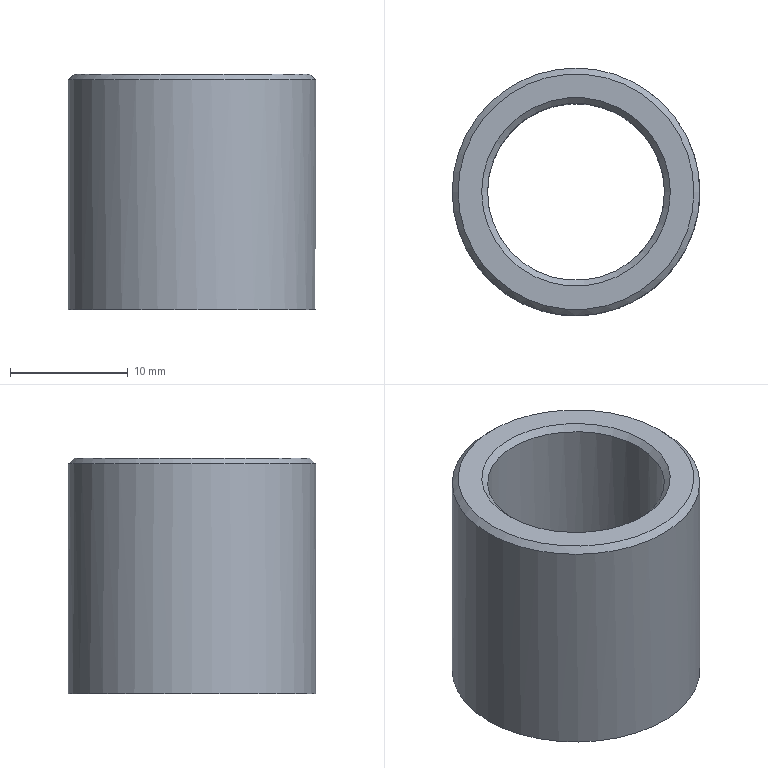Part | STEP file | Tube necking machine_id70_x_t | 1 solid | 6 faces | box 21 x 21 x 20 mm | volume 3379 mm3 | cylinder 2 | plane 2 | cone 2 | commonest cylinder face diameters 15 x1 21 x1
STEP:
#1=CARTESIAN_POINT('',(0.,0.,0.));
#2=DIRECTION('',(0.,0.,1.));
#3=DIRECTION('',(1.,0.,0.));
#4=AXIS2_PLACEMENT_3D('',#1,#2,#3);
#5=CARTESIAN_POINT('',(-39.5,90.,245.5));
#6=VERTEX_POINT('',#5);
#7=CARTESIAN_POINT('',(-60.5,90.,245.5));
#8=VERTEX_POINT('',#7);
#9=CARTESIAN_POINT('',(-50.,90.,245.5));
#10=DIRECTION('',(0.,0.,-1.));
#11=DIRECTION('',(1.,0.,0.));
#12=AXIS2_PLACEMENT_3D('',#9,#10,#11);
#13=CIRCLE('',#12,10.5);
#14=CARTESIAN_POINT('',(-50.,90.,226.));
#15=DIRECTION('',(0.,0.,1.));
#16=DIRECTION('',(-1.,0.,0.));
#17=AXIS2_PLACEMENT_3D('',#14,#15,#16);
#18=CYLINDRICAL_SURFACE('',#17,10.5);
#19=CARTESIAN_POINT('',(3.142,19.5));
#20=DIRECTION('',(-1.,0.));
#21=VECTOR('',#20,1.);
#22=LINE('',#19,#21);
#23=(GEOMETRIC_REPRESENTATION_CONTEXT(2)PARAMETRIC_REPRESENTATION_CONTEXT()REPRESENTATION_CONTEXT('',''));
#24=DEFINITIONAL_REPRESENTATION('',(#22),#23);
#25=PCURVE('',#18,#24);
#26=CARTESIAN_POINT('',(-50.,90.,246.));
#27=DIRECTION('',(0.,0.,-1.));
#28=DIRECTION('',(-1.,0.,0.));
#29=AXIS2_PLACEMENT_3D('',#26,#27,#28);
#30=CONICAL_SURFACE('',#29,10.,0.7854);
#31=CARTESIAN_POINT('',(3.142,0.5));
#32=DIRECTION('',(1.,0.));
#33=VECTOR('',#32,1.);
#34=LINE('',#31,#33);
#35=(GEOMETRIC_REPRESENTATION_CONTEXT(2)PARAMETRIC_REPRESENTATION_CONTEXT()REPRESENTATION_CONTEXT('',''));
#36=DEFINITIONAL_REPRESENTATION('',(#34),#35);
#37=PCURVE('',#30,#36);
#38=SURFACE_CURVE('',#13,(#25,#37),.PCURVE_S1.);
#39=EDGE_CURVE('',#6,#8,#38,.T.);
#40=ORIENTED_EDGE('',*,*,#39,.T.);
#41=CARTESIAN_POINT('',(-60.5,90.,226.));
#42=VERTEX_POINT('',#41);
#43=CARTESIAN_POINT('',(-60.5,90.,226.));
#44=CARTESIAN_POINT('',(-60.5,90.,245.5));
#45=B_SPLINE_CURVE_WITH_KNOTS('',1,(#43,#44),.UNSPECIFIED.,.F.,.F.,(2,2),(0.,19.5),.PIECEWISE_BEZIER_KNOTS.);
#46=CARTESIAN_POINT('',(0.,0.));
#47=DIRECTION('',(0.,1.));
#48=VECTOR('',#47,1.);
#49=LINE('',#46,#48);
#50=(GEOMETRIC_REPRESENTATION_CONTEXT(2)PARAMETRIC_REPRESENTATION_CONTEXT()REPRESENTATION_CONTEXT('',''));
#51=DEFINITIONAL_REPRESENTATION('',(#49),#50);
#52=PCURVE('',#18,#51);
#53=CARTESIAN_POINT('',(6.283,0.));
#54=DIRECTION('',(0.,1.));
#55=VECTOR('',#54,1.);
#56=LINE('',#53,#55);
#57=(GEOMETRIC_REPRESENTATION_CONTEXT(2)PARAMETRIC_REPRESENTATION_CONTEXT()REPRESENTATION_CONTEXT('',''));
#58=DEFINITIONAL_REPRESENTATION('',(#56),#57);
#59=PCURVE('',#18,#58);
#60=SEAM_CURVE('',#45,(#52,#59),.PCURVE_S1.);
#61=EDGE_CURVE('',#42,#8,#60,.T.);
#62=ORIENTED_EDGE('',*,*,#61,.F.);
#63=CARTESIAN_POINT('',(-50.,90.,226.));
#64=DIRECTION('',(0.,0.,1.));
#65=DIRECTION('',(-1.,0.,0.));
#66=AXIS2_PLACEMENT_3D('',#63,#64,#65);
#67=CIRCLE('',#66,10.5);
#68=CARTESIAN_POINT('',(0.,0.));
#69=DIRECTION('',(1.,0.));
#70=VECTOR('',#69,1.);
#71=LINE('',#68,#70);
#72=(GEOMETRIC_REPRESENTATION_CONTEXT(2)PARAMETRIC_REPRESENTATION_CONTEXT()REPRESENTATION_CONTEXT('',''));
#73=DEFINITIONAL_REPRESENTATION('',(#71),#72);
#74=PCURVE('',#18,#73);
#75=CARTESIAN_POINT('',(-50.,90.,226.));
#76=DIRECTION('',(0.,0.,1.));
#77=DIRECTION('',(-1.,0.,0.));
#78=AXIS2_PLACEMENT_3D('',#75,#76,#77);
#79=PLANE('',#78);
#80=CARTESIAN_POINT('',(0.,0.));
#81=DIRECTION('',(1.,0.));
#82=AXIS2_PLACEMENT_2D('',#80,#81);
#83=CIRCLE('',#82,10.5);
#84=(GEOMETRIC_REPRESENTATION_CONTEXT(2)PARAMETRIC_REPRESENTATION_CONTEXT()REPRESENTATION_CONTEXT('',''));
#85=DEFINITIONAL_REPRESENTATION('',(#83),#84);
#86=PCURVE('',#79,#85);
#87=SURFACE_CURVE('',#67,(#74,#86),.PCURVE_S1.);
#88=EDGE_CURVE('',#42,#42,#87,.T.);
#89=ORIENTED_EDGE('',*,*,#88,.T.);
#90=ORIENTED_EDGE('',*,*,#61,.T.);
#91=CARTESIAN_POINT('',(-50.,90.,245.5));
#92=DIRECTION('',(0.,0.,-1.));
#93=DIRECTION('',(1.,0.,0.));
#94=AXIS2_PLACEMENT_3D('',#91,#92,#93);
#95=CIRCLE('',#94,10.5);
#96=CARTESIAN_POINT('',(9.425,19.5));
#97=DIRECTION('',(-1.,0.));
#98=VECTOR('',#97,1.);
#99=LINE('',#96,#98);
#100=(GEOMETRIC_REPRESENTATION_CONTEXT(2)PARAMETRIC_REPRESENTATION_CONTEXT()REPRESENTATION_CONTEXT('',''));
#101=DEFINITIONAL_REPRESENTATION('',(#99),#100);
#102=PCURVE('',#18,#101);
#103=CARTESIAN_POINT('',(3.142,0.5));
#104=DIRECTION('',(1.,0.));
#105=VECTOR('',#104,1.);
#106=LINE('',#103,#105);
#107=(GEOMETRIC_REPRESENTATION_CONTEXT(2)PARAMETRIC_REPRESENTATION_CONTEXT()REPRESENTATION_CONTEXT('',''));
#108=DEFINITIONAL_REPRESENTATION('',(#106),#107);
#109=PCURVE('',#30,#108);
#110=SURFACE_CURVE('',#95,(#102,#109),.PCURVE_S1.);
#111=EDGE_CURVE('',#8,#6,#110,.T.);
#112=ORIENTED_EDGE('',*,*,#111,.T.);
#113=EDGE_LOOP('',(#40,#62,#89,#90,#112));
#114=FACE_BOUND('',#113,.T.);
#115=ADVANCED_FACE('',(#114),#18,.T.);
#116=CARTESIAN_POINT('',(-57.5,90.,245.5));
#117=VERTEX_POINT('',#116);
#118=CARTESIAN_POINT('',(-42.5,90.,245.5));
#119=VERTEX_POINT('',#118);
#120=CARTESIAN_POINT('',(-50.,90.,245.5));
#121=DIRECTION('',(0.,0.,1.));
#122=DIRECTION('',(1.,0.,0.));
#123=AXIS2_PLACEMENT_3D('',#120,#121,#122);
#124=CIRCLE('',#123,7.5);
#125=CARTESIAN_POINT('',(-50.,90.,226.));
#126=DIRECTION('',(0.,0.,1.));
#127=DIRECTION('',(-1.,0.,0.));
#128=AXIS2_PLACEMENT_3D('',#125,#126,#127);
#129=CYLINDRICAL_SURFACE('',#128,7.5);
#130=CARTESIAN_POINT('',(-3.142,19.5));
#131=DIRECTION('',(1.,0.));
#132=VECTOR('',#131,1.);
#133=LINE('',#130,#132);
#134=(GEOMETRIC_REPRESENTATION_CONTEXT(2)PARAMETRIC_REPRESENTATION_CONTEXT()REPRESENTATION_CONTEXT('',''));
#135=DEFINITIONAL_REPRESENTATION('',(#133),#134);
#136=PCURVE('',#129,#135);
#137=CARTESIAN_POINT('',(-50.,90.,245.5));
#138=DIRECTION('',(0.,0.,1.));
#139=DIRECTION('',(1.,0.,0.));
#140=AXIS2_PLACEMENT_3D('',#137,#138,#139);
#141=CONICAL_SURFACE('',#140,7.5,0.7854);
#142=CARTESIAN_POINT('',(0.,0.));
#143=DIRECTION('',(1.,0.));
#144=VECTOR('',#143,1.);
#145=LINE('',#142,#144);
#146=(GEOMETRIC_REPRESENTATION_CONTEXT(2)PARAMETRIC_REPRESENTATION_CONTEXT()REPRESENTATION_CONTEXT('',''));
#147=DEFINITIONAL_REPRESENTATION('',(#145),#146);
#148=PCURVE('',#141,#147);
#149=SURFACE_CURVE('',#124,(#136,#148),.PCURVE_S1.);
#150=EDGE_CURVE('',#117,#119,#149,.T.);
#151=ORIENTED_EDGE('',*,*,#150,.F.);
#152=CARTESIAN_POINT('',(-57.5,90.,226.));
#153=VERTEX_POINT('',#152);
#154=CARTESIAN_POINT('',(-57.5,90.,226.));
#155=CARTESIAN_POINT('',(-57.5,90.,245.5));
#156=B_SPLINE_CURVE_WITH_KNOTS('',1,(#154,#155),.UNSPECIFIED.,.F.,.F.,(2,2),(0.,19.5),.PIECEWISE_BEZIER_KNOTS.);
#157=CARTESIAN_POINT('',(0.,0.));
#158=DIRECTION('',(0.,1.));
#159=VECTOR('',#158,1.);
#160=LINE('',#157,#159);
#161=(GEOMETRIC_REPRESENTATION_CONTEXT(2)PARAMETRIC_REPRESENTATION_CONTEXT()REPRESENTATION_CONTEXT('',''));
#162=DEFINITIONAL_REPRESENTATION('',(#160),#161);
#163=PCURVE('',#129,#162);
#164=CARTESIAN_POINT('',(6.283,0.));
#165=DIRECTION('',(0.,1.));
#166=VECTOR('',#165,1.);
#167=LINE('',#164,#166);
#168=(GEOMETRIC_REPRESENTATION_CONTEXT(2)PARAMETRIC_REPRESENTATION_CONTEXT()REPRESENTATION_CONTEXT('',''));
#169=DEFINITIONAL_REPRESENTATION('',(#167),#168);
#170=PCURVE('',#129,#169);
#171=SEAM_CURVE('',#156,(#163,#170),.PCURVE_S1.);
#172=EDGE_CURVE('',#153,#117,#171,.T.);
#173=ORIENTED_EDGE('',*,*,#172,.F.);
#174=CARTESIAN_POINT('',(-50.,90.,226.));
#175=DIRECTION('',(0.,0.,1.));
#176=DIRECTION('',(-1.,0.,0.));
#177=AXIS2_PLACEMENT_3D('',#174,#175,#176);
#178=CIRCLE('',#177,7.5);
#179=CARTESIAN_POINT('',(0.,0.));
#180=DIRECTION('',(1.,0.));
#181=VECTOR('',#180,1.);
#182=LINE('',#179,#181);
#183=(GEOMETRIC_REPRESENTATION_CONTEXT(2)PARAMETRIC_REPRESENTATION_CONTEXT()REPRESENTATION_CONTEXT('',''));
#184=DEFINITIONAL_REPRESENTATION('',(#182),#183);
#185=PCURVE('',#129,#184);
#186=CARTESIAN_POINT('',(0.,0.));
#187=DIRECTION('',(1.,0.));
#188=AXIS2_PLACEMENT_2D('',#186,#187);
#189=CIRCLE('',#188,7.5);
#190=(GEOMETRIC_REPRESENTATION_CONTEXT(2)PARAMETRIC_REPRESENTATION_CONTEXT()REPRESENTATION_CONTEXT('',''));
#191=DEFINITIONAL_REPRESENTATION('',(#189),#190);
#192=PCURVE('',#79,#191);
#193=SURFACE_CURVE('',#178,(#185,#192),.PCURVE_S1.);
#194=EDGE_CURVE('',#153,#153,#193,.T.);
#195=ORIENTED_EDGE('',*,*,#194,.T.);
#196=ORIENTED_EDGE('',*,*,#172,.T.);
#197=CARTESIAN_POINT('',(-50.,90.,245.5));
#198=DIRECTION('',(0.,0.,1.));
#199=DIRECTION('',(1.,0.,0.));
#200=AXIS2_PLACEMENT_3D('',#197,#198,#199);
#201=CIRCLE('',#200,7.5);
#202=CARTESIAN_POINT('',(3.142,19.5));
#203=DIRECTION('',(1.,0.));
#204=VECTOR('',#203,1.);
#205=LINE('',#202,#204);
#206=(GEOMETRIC_REPRESENTATION_CONTEXT(2)PARAMETRIC_REPRESENTATION_CONTEXT()REPRESENTATION_CONTEXT('',''));
#207=DEFINITIONAL_REPRESENTATION('',(#205),#206);
#208=PCURVE('',#129,#207);
#209=CARTESIAN_POINT('',(0.,0.));
#210=DIRECTION('',(1.,0.));
#211=VECTOR('',#210,1.);
#212=LINE('',#209,#211);
#213=(GEOMETRIC_REPRESENTATION_CONTEXT(2)PARAMETRIC_REPRESENTATION_CONTEXT()REPRESENTATION_CONTEXT('',''));
#214=DEFINITIONAL_REPRESENTATION('',(#212),#213);
#215=PCURVE('',#141,#214);
#216=SURFACE_CURVE('',#201,(#208,#215),.PCURVE_S1.);
#217=EDGE_CURVE('',#119,#117,#216,.T.);
#218=ORIENTED_EDGE('',*,*,#217,.F.);
#219=EDGE_LOOP('',(#151,#173,#195,#196,#218));
#220=FACE_BOUND('',#219,.F.);
#221=ADVANCED_FACE('',(#220),#129,.F.);
#222=ORIENTED_EDGE('',*,*,#88,.F.);
#223=EDGE_LOOP('',(#222));
#224=FACE_BOUND('',#223,.T.);
#225=ORIENTED_EDGE('',*,*,#194,.T.);
#226=EDGE_LOOP('',(#225));
#227=FACE_BOUND('',#226,.T.);
#228=ADVANCED_FACE('',(#224,#227),#79,.F.);
#229=CARTESIAN_POINT('',(-40.,90.,246.));
#230=VERTEX_POINT('',#229);
#231=CARTESIAN_POINT('',(-50.,90.,246.));
#232=DIRECTION('',(0.,0.,1.));
#233=DIRECTION('',(1.,0.,0.));
#234=AXIS2_PLACEMENT_3D('',#231,#232,#233);
#235=CIRCLE('',#234,10.);
#236=CARTESIAN_POINT('',(-50.,90.,246.));
#237=DIRECTION('',(0.,0.,1.));
#238=DIRECTION('',(-1.,0.,0.));
#239=AXIS2_PLACEMENT_3D('',#236,#237,#238);
#240=PLANE('',#239);
#241=CARTESIAN_POINT('',(0.,0.));
#242=DIRECTION('',(-1.,0.));
#243=AXIS2_PLACEMENT_2D('',#241,#242);
#244=CIRCLE('',#243,10.);
#245=(GEOMETRIC_REPRESENTATION_CONTEXT(2)PARAMETRIC_REPRESENTATION_CONTEXT()REPRESENTATION_CONTEXT('',''));
#246=DEFINITIONAL_REPRESENTATION('',(#244),#245);
#247=PCURVE('',#240,#246);
#248=CARTESIAN_POINT('',(9.425,0.));
#249=DIRECTION('',(-1.,0.));
#250=VECTOR('',#249,1.);
#251=LINE('',#248,#250);
#252=(GEOMETRIC_REPRESENTATION_CONTEXT(2)PARAMETRIC_REPRESENTATION_CONTEXT()REPRESENTATION_CONTEXT('',''));
#253=DEFINITIONAL_REPRESENTATION('',(#251),#252);
#254=PCURVE('',#30,#253);
#255=SURFACE_CURVE('',#235,(#247,#254),.PCURVE_S1.);
#256=EDGE_CURVE('',#230,#230,#255,.T.);
#257=ORIENTED_EDGE('',*,*,#256,.T.);
#258=EDGE_LOOP('',(#257));
#259=FACE_BOUND('',#258,.T.);
#260=CARTESIAN_POINT('',(-42.,90.,246.));
#261=VERTEX_POINT('',#260);
#262=CARTESIAN_POINT('',(-50.,90.,246.));
#263=DIRECTION('',(0.,0.,-1.));
#264=DIRECTION('',(1.,0.,0.));
#265=AXIS2_PLACEMENT_3D('',#262,#263,#264);
#266=CIRCLE('',#265,8.);
#267=CARTESIAN_POINT('',(-8.,0.));
#268=CARTESIAN_POINT('',(-8.,13.856));
#269=CARTESIAN_POINT('',(4.,6.928));
#270=CARTESIAN_POINT('',(16.,0.));
#271=CARTESIAN_POINT('',(4.,-6.928));
#272=CARTESIAN_POINT('',(-8.,-13.856));
#273=CARTESIAN_POINT('',(-8.,0.));
#274=(BOUNDED_CURVE()B_SPLINE_CURVE(2,(#267,#268,#269,#270,#271,#272,#273),.UNSPECIFIED.,.T.,.F.)B_SPLINE_CURVE_WITH_KNOTS((1,2,2,2,2,1),(-2.094,0.,2.094,4.189,6.283,8.378),.UNSPECIFIED.)CURVE()GEOMETRIC_REPRESENTATION_ITEM()RATIONAL_B_SPLINE_CURVE((1.,0.5,1.,0.5,1.,0.5,1.))REPRESENTATION_ITEM(''));
#275=(GEOMETRIC_REPRESENTATION_CONTEXT(2)PARAMETRIC_REPRESENTATION_CONTEXT()REPRESENTATION_CONTEXT('',''));
#276=DEFINITIONAL_REPRESENTATION('',(#274),#275);
#277=PCURVE('',#240,#276);
#278=CARTESIAN_POINT('',(6.283,0.5));
#279=DIRECTION('',(-1.,0.));
#280=VECTOR('',#279,1.);
#281=LINE('',#278,#280);
#282=(GEOMETRIC_REPRESENTATION_CONTEXT(2)PARAMETRIC_REPRESENTATION_CONTEXT()REPRESENTATION_CONTEXT('',''));
#283=DEFINITIONAL_REPRESENTATION('',(#281),#282);
#284=PCURVE('',#141,#283);
#285=SURFACE_CURVE('',#266,(#277,#284),.PCURVE_S1.);
#286=EDGE_CURVE('',#261,#261,#285,.T.);
#287=ORIENTED_EDGE('',*,*,#286,.T.);
#288=EDGE_LOOP('',(#287));
#289=FACE_BOUND('',#288,.T.);
#290=ADVANCED_FACE('',(#259,#289),#240,.T.);
#291=ORIENTED_EDGE('',*,*,#286,.T.);
#292=CARTESIAN_POINT('',(-42.5,90.,245.5));
#293=CARTESIAN_POINT('',(-42.,90.,246.));
#294=B_SPLINE_CURVE_WITH_KNOTS('',1,(#292,#293),.UNSPECIFIED.,.F.,.F.,(2,2),(0.,0.7071),.PIECEWISE_BEZIER_KNOTS.);
#295=CARTESIAN_POINT('',(0.,0.));
#296=DIRECTION('',(0.,1.));
#297=VECTOR('',#296,1.);
#298=LINE('',#295,#297);
#299=(GEOMETRIC_REPRESENTATION_CONTEXT(2)PARAMETRIC_REPRESENTATION_CONTEXT()REPRESENTATION_CONTEXT('',''));
#300=DEFINITIONAL_REPRESENTATION('',(#298),#299);
#301=PCURVE('',#141,#300);
#302=CARTESIAN_POINT('',(6.283,0.));
#303=DIRECTION('',(0.,1.));
#304=VECTOR('',#303,1.);
#305=LINE('',#302,#304);
#306=(GEOMETRIC_REPRESENTATION_CONTEXT(2)PARAMETRIC_REPRESENTATION_CONTEXT()REPRESENTATION_CONTEXT('',''));
#307=DEFINITIONAL_REPRESENTATION('',(#305),#306);
#308=PCURVE('',#141,#307);
#309=SEAM_CURVE('',#294,(#301,#308),.PCURVE_S1.);
#310=EDGE_CURVE('',#119,#261,#309,.T.);
#311=ORIENTED_EDGE('',*,*,#310,.F.);
#312=ORIENTED_EDGE('',*,*,#217,.T.);
#313=ORIENTED_EDGE('',*,*,#150,.T.);
#314=ORIENTED_EDGE('',*,*,#310,.T.);
#315=EDGE_LOOP('',(#291,#311,#312,#313,#314));
#316=FACE_BOUND('',#315,.F.);
#317=ADVANCED_FACE('',(#316),#141,.F.);
#318=ORIENTED_EDGE('',*,*,#39,.F.);
#319=CARTESIAN_POINT('',(-40.,90.,246.));
#320=CARTESIAN_POINT('',(-39.5,90.,245.5));
#321=B_SPLINE_CURVE_WITH_KNOTS('',1,(#319,#320),.UNSPECIFIED.,.F.,.F.,(2,2),(0.,0.7071),.PIECEWISE_BEZIER_KNOTS.);
#322=CARTESIAN_POINT('',(3.142,0.));
#323=DIRECTION('',(0.,1.));
#324=VECTOR('',#323,1.);
#325=LINE('',#322,#324);
#326=(GEOMETRIC_REPRESENTATION_CONTEXT(2)PARAMETRIC_REPRESENTATION_CONTEXT()REPRESENTATION_CONTEXT('',''));
#327=DEFINITIONAL_REPRESENTATION('',(#325),#326);
#328=PCURVE('',#30,#327);
#329=CARTESIAN_POINT('',(9.425,0.));
#330=DIRECTION('',(0.,1.));
#331=VECTOR('',#330,1.);
#332=LINE('',#329,#331);
#333=(GEOMETRIC_REPRESENTATION_CONTEXT(2)PARAMETRIC_REPRESENTATION_CONTEXT()REPRESENTATION_CONTEXT('',''));
#334=DEFINITIONAL_REPRESENTATION('',(#332),#333);
#335=PCURVE('',#30,#334);
#336=SEAM_CURVE('',#321,(#328,#335),.PCURVE_S1.);
#337=EDGE_CURVE('',#230,#6,#336,.T.);
#338=ORIENTED_EDGE('',*,*,#337,.F.);
#339=ORIENTED_EDGE('',*,*,#256,.F.);
#340=ORIENTED_EDGE('',*,*,#337,.T.);
#341=ORIENTED_EDGE('',*,*,#111,.F.);
#342=EDGE_LOOP('',(#318,#338,#339,#340,#341));
#343=FACE_BOUND('',#342,.T.);
#344=ADVANCED_FACE('',(#343),#30,.T.);
#345=CLOSED_SHELL('',(#115,#221,#228,#290,#317,#344));
#346=MANIFOLD_SOLID_BREP('',#345);
#347=(LENGTH_UNIT()NAMED_UNIT(*)SI_UNIT(.MILLI.,.METRE.));
#348=UNCERTAINTY_MEASURE_WITH_UNIT(LENGTH_MEASURE(0.00001),#347,'','');
#349=(NAMED_UNIT(*)PLANE_ANGLE_UNIT()SI_UNIT($,.RADIAN.));
#350=(NAMED_UNIT(*)SI_UNIT($,.STERADIAN.)SOLID_ANGLE_UNIT());
#351=(GEOMETRIC_REPRESENTATION_CONTEXT(3)GLOBAL_UNCERTAINTY_ASSIGNED_CONTEXT((#348))GLOBAL_UNIT_ASSIGNED_CONTEXT((#347,#349,#350))REPRESENTATION_CONTEXT('',''));
#352=ADVANCED_BREP_SHAPE_REPRESENTATION('',(#4,#346),#351);